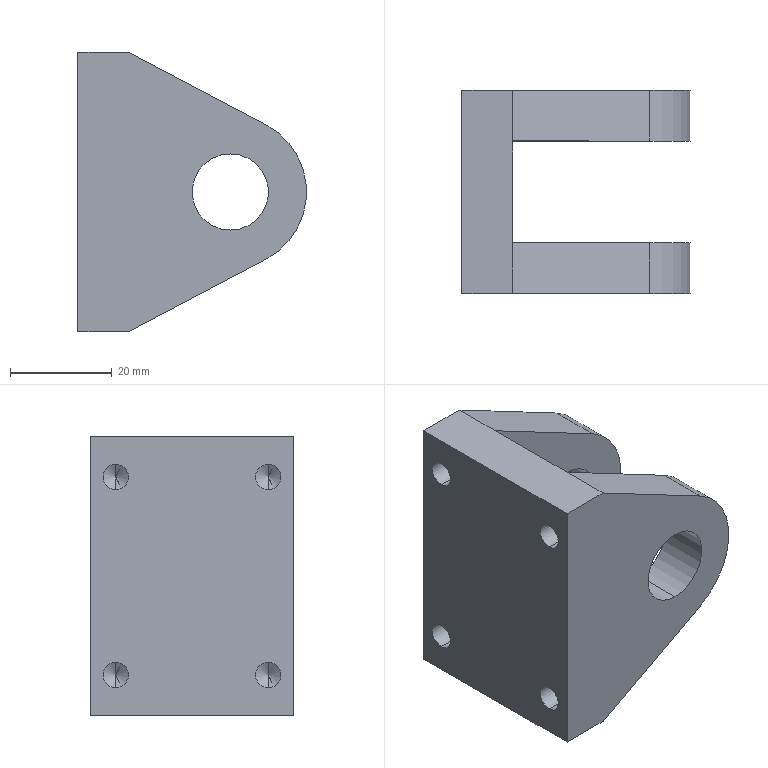Part | SolidWorks | features Chamfer 1, Extrusion 1, HoleWzd 1, ICE 1 | 1 solid | 34 faces | box 45 x 40 x 55 mm | volume 42289 mm3 | cylinder 14 | plane 12 | cone 8 | commonest cylinder face diameters 5 x8 15 x4 30 x2
STEP:
#1=CARTESIAN_POINT('',(15.,5.,-22.));
#2=VERTEX_POINT('',#1);
#3=CARTESIAN_POINT('',(15.,5.,-17.));
#4=VERTEX_POINT('',#3);
#5=CARTESIAN_POINT('',(15.,5.,-19.5));
#6=DIRECTION('',(-1.,0.,0.));
#7=DIRECTION('',(0.,0.,1.));
#8=AXIS2_PLACEMENT_3D('',#5,#6,#7);
#9=CIRCLE('',#8,2.5);
#10=EDGE_CURVE('',#2,#4,#9,.T.);
#11=ORIENTED_EDGE('',*,*,#10,.F.);
#12=CARTESIAN_POINT('',(0.,5.,-22.));
#13=VERTEX_POINT('',#12);
#14=CARTESIAN_POINT('',(0.,5.,-22.));
#15=DIRECTION('',(-1.,0.,0.));
#16=VECTOR('',#15,1000.);
#17=LINE('',#14,#16);
#18=EDGE_CURVE('',#2,#13,#17,.T.);
#19=ORIENTED_EDGE('',*,*,#18,.T.);
#20=CARTESIAN_POINT('',(0.,5.,-17.));
#21=VERTEX_POINT('',#20);
#22=CARTESIAN_POINT('',(0.,5.,-19.5));
#23=DIRECTION('',(-1.,0.,0.));
#24=DIRECTION('',(0.,0.,1.));
#25=AXIS2_PLACEMENT_3D('',#22,#23,#24);
#26=CIRCLE('',#25,2.5);
#27=EDGE_CURVE('',#13,#21,#26,.T.);
#28=ORIENTED_EDGE('',*,*,#27,.T.);
#29=CARTESIAN_POINT('',(0.,5.,-17.));
#30=DIRECTION('',(-1.,0.,0.));
#31=VECTOR('',#30,1000.);
#32=LINE('',#29,#31);
#33=EDGE_CURVE('',#4,#21,#32,.T.);
#34=ORIENTED_EDGE('',*,*,#33,.F.);
#35=EDGE_LOOP('',(#11,#19,#28,#34));
#36=FACE_OUTER_BOUND('',#35,.T.);
#37=CARTESIAN_POINT('',(0.,5.,-19.5));
#38=DIRECTION('',(-1.,0.,0.));
#39=DIRECTION('',(0.,0.,1.));
#40=AXIS2_PLACEMENT_3D('',#37,#38,#39);
#41=CYLINDRICAL_SURFACE('',#40,2.5);
#42=ADVANCED_FACE('',(#36),#41,.F.);
#43=CARTESIAN_POINT('',(16.502,5.,-19.5));
#44=VERTEX_POINT('',#43);
#45=CARTESIAN_POINT('',(15.,5.,-17.));
#46=DIRECTION('',(-0.515,0.,0.8572));
#47=VECTOR('',#46,1000.);
#48=LINE('',#45,#47);
#49=EDGE_CURVE('',#44,#4,#48,.T.);
#50=ORIENTED_EDGE('',*,*,#49,.F.);
#51=CARTESIAN_POINT('',(15.,5.,-22.));
#52=DIRECTION('',(-0.515,0.,-0.8572));
#53=VECTOR('',#52,1000.);
#54=LINE('',#51,#53);
#55=EDGE_CURVE('',#44,#2,#54,.T.);
#56=ORIENTED_EDGE('',*,*,#55,.T.);
#57=ORIENTED_EDGE('',*,*,#10,.T.);
#58=EDGE_LOOP('',(#50,#56,#57));
#59=FACE_OUTER_BOUND('',#58,.T.);
#60=CARTESIAN_POINT('',(15.,5.,-19.5));
#61=DIRECTION('',(-1.,0.,0.));
#62=DIRECTION('',(0.,0.,1.));
#63=AXIS2_PLACEMENT_3D('',#60,#61,#62);
#64=CONICAL_SURFACE('',#63,2.5,1.03);
#65=ADVANCED_FACE('',(#59),#64,.F.);
#66=CARTESIAN_POINT('',(15.,35.,-22.));
#67=VERTEX_POINT('',#66);
#68=CARTESIAN_POINT('',(15.,35.,-17.));
#69=VERTEX_POINT('',#68);
#70=CARTESIAN_POINT('',(15.,35.,-19.5));
#71=DIRECTION('',(-1.,0.,0.));
#72=DIRECTION('',(0.,0.,1.));
#73=AXIS2_PLACEMENT_3D('',#70,#71,#72);
#74=CIRCLE('',#73,2.5);
#75=EDGE_CURVE('',#67,#69,#74,.T.);
#76=ORIENTED_EDGE('',*,*,#75,.F.);
#77=CARTESIAN_POINT('',(0.,35.,-22.));
#78=VERTEX_POINT('',#77);
#79=CARTESIAN_POINT('',(0.,35.,-22.));
#80=DIRECTION('',(-1.,0.,0.));
#81=VECTOR('',#80,1000.);
#82=LINE('',#79,#81);
#83=EDGE_CURVE('',#67,#78,#82,.T.);
#84=ORIENTED_EDGE('',*,*,#83,.T.);
#85=CARTESIAN_POINT('',(0.,35.,-17.));
#86=VERTEX_POINT('',#85);
#87=CARTESIAN_POINT('',(0.,35.,-19.5));
#88=DIRECTION('',(-1.,0.,0.));
#89=DIRECTION('',(0.,0.,1.));
#90=AXIS2_PLACEMENT_3D('',#87,#88,#89);
#91=CIRCLE('',#90,2.5);
#92=EDGE_CURVE('',#78,#86,#91,.T.);
#93=ORIENTED_EDGE('',*,*,#92,.T.);
#94=CARTESIAN_POINT('',(0.,35.,-17.));
#95=DIRECTION('',(-1.,0.,0.));
#96=VECTOR('',#95,1000.);
#97=LINE('',#94,#96);
#98=EDGE_CURVE('',#69,#86,#97,.T.);
#99=ORIENTED_EDGE('',*,*,#98,.F.);
#100=EDGE_LOOP('',(#76,#84,#93,#99));
#101=FACE_OUTER_BOUND('',#100,.T.);
#102=CARTESIAN_POINT('',(0.,35.,-19.5));
#103=DIRECTION('',(-1.,0.,0.));
#104=DIRECTION('',(0.,0.,1.));
#105=AXIS2_PLACEMENT_3D('',#102,#103,#104);
#106=CYLINDRICAL_SURFACE('',#105,2.5);
#107=ADVANCED_FACE('',(#101),#106,.F.);
#108=CARTESIAN_POINT('',(16.502,35.,-19.5));
#109=VERTEX_POINT('',#108);
#110=CARTESIAN_POINT('',(15.,35.,-17.));
#111=DIRECTION('',(-0.515,0.,0.8572));
#112=VECTOR('',#111,1000.);
#113=LINE('',#110,#112);
#114=EDGE_CURVE('',#109,#69,#113,.T.);
#115=ORIENTED_EDGE('',*,*,#114,.F.);
#116=CARTESIAN_POINT('',(15.,35.,-22.));
#117=DIRECTION('',(-0.515,0.,-0.8572));
#118=VECTOR('',#117,1000.);
#119=LINE('',#116,#118);
#120=EDGE_CURVE('',#109,#67,#119,.T.);
#121=ORIENTED_EDGE('',*,*,#120,.T.);
#122=ORIENTED_EDGE('',*,*,#75,.T.);
#123=EDGE_LOOP('',(#115,#121,#122));
#124=FACE_OUTER_BOUND('',#123,.T.);
#125=CARTESIAN_POINT('',(15.,35.,-19.5));
#126=DIRECTION('',(-1.,0.,0.));
#127=DIRECTION('',(0.,0.,1.));
#128=AXIS2_PLACEMENT_3D('',#125,#126,#127);
#129=CONICAL_SURFACE('',#128,2.5,1.03);
#130=ADVANCED_FACE('',(#124),#129,.F.);
#131=CARTESIAN_POINT('',(15.,5.,17.));
#132=VERTEX_POINT('',#131);
#133=CARTESIAN_POINT('',(15.,5.,22.));
#134=VERTEX_POINT('',#133);
#135=CARTESIAN_POINT('',(15.,5.,19.5));
#136=DIRECTION('',(-1.,0.,0.));
#137=DIRECTION('',(0.,0.,1.));
#138=AXIS2_PLACEMENT_3D('',#135,#136,#137);
#139=CIRCLE('',#138,2.5);
#140=EDGE_CURVE('',#132,#134,#139,.T.);
#141=ORIENTED_EDGE('',*,*,#140,.F.);
#142=CARTESIAN_POINT('',(0.,5.,17.));
#143=VERTEX_POINT('',#142);
#144=CARTESIAN_POINT('',(0.,5.,17.));
#145=DIRECTION('',(-1.,0.,0.));
#146=VECTOR('',#145,1000.);
#147=LINE('',#144,#146);
#148=EDGE_CURVE('',#132,#143,#147,.T.);
#149=ORIENTED_EDGE('',*,*,#148,.T.);
#150=CARTESIAN_POINT('',(0.,5.,22.));
#151=VERTEX_POINT('',#150);
#152=CARTESIAN_POINT('',(0.,5.,19.5));
#153=DIRECTION('',(-1.,0.,0.));
#154=DIRECTION('',(0.,0.,1.));
#155=AXIS2_PLACEMENT_3D('',#152,#153,#154);
#156=CIRCLE('',#155,2.5);
#157=EDGE_CURVE('',#143,#151,#156,.T.);
#158=ORIENTED_EDGE('',*,*,#157,.T.);
#159=CARTESIAN_POINT('',(0.,5.,22.));
#160=DIRECTION('',(-1.,0.,0.));
#161=VECTOR('',#160,1000.);
#162=LINE('',#159,#161);
#163=EDGE_CURVE('',#134,#151,#162,.T.);
#164=ORIENTED_EDGE('',*,*,#163,.F.);
#165=EDGE_LOOP('',(#141,#149,#158,#164));
#166=FACE_OUTER_BOUND('',#165,.T.);
#167=CARTESIAN_POINT('',(0.,5.,19.5));
#168=DIRECTION('',(-1.,0.,0.));
#169=DIRECTION('',(0.,0.,1.));
#170=AXIS2_PLACEMENT_3D('',#167,#168,#169);
#171=CYLINDRICAL_SURFACE('',#170,2.5);
#172=ADVANCED_FACE('',(#166),#171,.F.);
#173=CARTESIAN_POINT('',(16.502,5.,19.5));
#174=VERTEX_POINT('',#173);
#175=CARTESIAN_POINT('',(15.,5.,22.));
#176=DIRECTION('',(-0.515,0.,0.8572));
#177=VECTOR('',#176,1000.);
#178=LINE('',#175,#177);
#179=EDGE_CURVE('',#174,#134,#178,.T.);
#180=ORIENTED_EDGE('',*,*,#179,.F.);
#181=CARTESIAN_POINT('',(15.,5.,17.));
#182=DIRECTION('',(-0.515,0.,-0.8572));
#183=VECTOR('',#182,1000.);
#184=LINE('',#181,#183);
#185=EDGE_CURVE('',#174,#132,#184,.T.);
#186=ORIENTED_EDGE('',*,*,#185,.T.);
#187=ORIENTED_EDGE('',*,*,#140,.T.);
#188=EDGE_LOOP('',(#180,#186,#187));
#189=FACE_OUTER_BOUND('',#188,.T.);
#190=CARTESIAN_POINT('',(15.,5.,19.5));
#191=DIRECTION('',(-1.,0.,0.));
#192=DIRECTION('',(0.,0.,1.));
#193=AXIS2_PLACEMENT_3D('',#190,#191,#192);
#194=CONICAL_SURFACE('',#193,2.5,1.03);
#195=ADVANCED_FACE('',(#189),#194,.F.);
#196=CARTESIAN_POINT('',(15.,35.,17.));
#197=VERTEX_POINT('',#196);
#198=CARTESIAN_POINT('',(15.,35.,22.));
#199=VERTEX_POINT('',#198);
#200=CARTESIAN_POINT('',(15.,35.,19.5));
#201=DIRECTION('',(-1.,0.,0.));
#202=DIRECTION('',(0.,0.,1.));
#203=AXIS2_PLACEMENT_3D('',#200,#201,#202);
#204=CIRCLE('',#203,2.5);
#205=EDGE_CURVE('',#197,#199,#204,.T.);
#206=ORIENTED_EDGE('',*,*,#205,.F.);
#207=CARTESIAN_POINT('',(0.,35.,17.));
#208=VERTEX_POINT('',#207);
#209=CARTESIAN_POINT('',(0.,35.,17.));
#210=DIRECTION('',(-1.,0.,0.));
#211=VECTOR('',#210,1000.);
#212=LINE('',#209,#211);
#213=EDGE_CURVE('',#197,#208,#212,.T.);
#214=ORIENTED_EDGE('',*,*,#213,.T.);
#215=CARTESIAN_POINT('',(0.,35.,22.));
#216=VERTEX_POINT('',#215);
#217=CARTESIAN_POINT('',(0.,35.,19.5));
#218=DIRECTION('',(-1.,0.,0.));
#219=DIRECTION('',(0.,0.,1.));
#220=AXIS2_PLACEMENT_3D('',#217,#218,#219);
#221=CIRCLE('',#220,2.5);
#222=EDGE_CURVE('',#208,#216,#221,.T.);
#223=ORIENTED_EDGE('',*,*,#222,.T.);
#224=CARTESIAN_POINT('',(0.,35.,22.));
#225=DIRECTION('',(-1.,0.,0.));
#226=VECTOR('',#225,1000.);
#227=LINE('',#224,#226);
#228=EDGE_CURVE('',#199,#216,#227,.T.);
#229=ORIENTED_EDGE('',*,*,#228,.F.);
#230=EDGE_LOOP('',(#206,#214,#223,#229));
#231=FACE_OUTER_BOUND('',#230,.T.);
#232=CARTESIAN_POINT('',(0.,35.,19.5));
#233=DIRECTION('',(-1.,0.,0.));
#234=DIRECTION('',(0.,0.,1.));
#235=AXIS2_PLACEMENT_3D('',#232,#233,#234);
#236=CYLINDRICAL_SURFACE('',#235,2.5);
#237=ADVANCED_FACE('',(#231),#236,.F.);
#238=CARTESIAN_POINT('',(16.502,35.,19.5));
#239=VERTEX_POINT('',#238);
#240=CARTESIAN_POINT('',(15.,35.,22.));
#241=DIRECTION('',(-0.515,0.,0.8572));
#242=VECTOR('',#241,1000.);
#243=LINE('',#240,#242);
#244=EDGE_CURVE('',#239,#199,#243,.T.);
#245=ORIENTED_EDGE('',*,*,#244,.F.);
#246=CARTESIAN_POINT('',(15.,35.,17.));
#247=DIRECTION('',(-0.515,0.,-0.8572));
#248=VECTOR('',#247,1000.);
#249=LINE('',#246,#248);
#250=EDGE_CURVE('',#239,#197,#249,.T.);
#251=ORIENTED_EDGE('',*,*,#250,.T.);
#252=ORIENTED_EDGE('',*,*,#205,.T.);
#253=EDGE_LOOP('',(#245,#251,#252));
#254=FACE_OUTER_BOUND('',#253,.T.);
#255=CARTESIAN_POINT('',(15.,35.,19.5));
#256=DIRECTION('',(-1.,0.,0.));
#257=DIRECTION('',(0.,0.,1.));
#258=AXIS2_PLACEMENT_3D('',#255,#256,#257);
#259=CONICAL_SURFACE('',#258,2.5,1.03);
#260=ADVANCED_FACE('',(#254),#259,.F.);
#261=CARTESIAN_POINT('',(30.,40.,-7.5));
#262=VERTEX_POINT('',#261);
#263=CARTESIAN_POINT('',(30.,40.,7.5));
#264=VERTEX_POINT('',#263);
#265=CARTESIAN_POINT('',(30.,40.,0.));
#266=DIRECTION('',(0.,1.,0.));
#267=DIRECTION('',(0.,0.,1.));
#268=AXIS2_PLACEMENT_3D('',#265,#266,#267);
#269=CIRCLE('',#268,7.5);
#270=EDGE_CURVE('',#262,#264,#269,.T.);
#271=ORIENTED_EDGE('',*,*,#270,.T.);
#272=CARTESIAN_POINT('',(30.,30.,7.5));
#273=VERTEX_POINT('',#272);
#274=CARTESIAN_POINT('',(30.,40.,7.5));
#275=DIRECTION('',(0.,-1.,0.));
#276=VECTOR('',#275,1000.);
#277=LINE('',#274,#276);
#278=EDGE_CURVE('',#264,#273,#277,.T.);
#279=ORIENTED_EDGE('',*,*,#278,.T.);
#280=CARTESIAN_POINT('',(30.,30.,-7.5));
#281=VERTEX_POINT('',#280);
#282=CARTESIAN_POINT('',(30.,30.,0.));
#283=DIRECTION('',(0.,1.,0.));
#284=DIRECTION('',(-1.,0.,0.));
#285=AXIS2_PLACEMENT_3D('',#282,#283,#284);
#286=CIRCLE('',#285,7.5);
#287=EDGE_CURVE('',#281,#273,#286,.T.);
#288=ORIENTED_EDGE('',*,*,#287,.F.);
#289=CARTESIAN_POINT('',(30.,40.,-7.5));
#290=DIRECTION('',(0.,-1.,0.));
#291=VECTOR('',#290,1000.);
#292=LINE('',#289,#291);
#293=EDGE_CURVE('',#262,#281,#292,.T.);
#294=ORIENTED_EDGE('',*,*,#293,.F.);
#295=EDGE_LOOP('',(#271,#279,#288,#294));
#296=FACE_OUTER_BOUND('',#295,.T.);
#297=CARTESIAN_POINT('',(30.,40.,0.));
#298=DIRECTION('',(0.,-1.,0.));
#299=DIRECTION('',(0.,0.,-1.));
#300=AXIS2_PLACEMENT_3D('',#297,#298,#299);
#301=CYLINDRICAL_SURFACE('',#300,7.5);
#302=ADVANCED_FACE('',(#296),#301,.F.);
#303=CARTESIAN_POINT('',(30.,10.,7.5));
#304=VERTEX_POINT('',#303);
#305=CARTESIAN_POINT('',(30.,10.,-7.5));
#306=VERTEX_POINT('',#305);
#307=CARTESIAN_POINT('',(30.,10.,0.));
#308=DIRECTION('',(0.,-1.,0.));
#309=DIRECTION('',(1.,0.,0.));
#310=AXIS2_PLACEMENT_3D('',#307,#308,#309);
#311=CIRCLE('',#310,7.5);
#312=EDGE_CURVE('',#304,#306,#311,.T.);
#313=ORIENTED_EDGE('',*,*,#312,.F.);
#314=CARTESIAN_POINT('',(30.,0.,7.5));
#315=VERTEX_POINT('',#314);
#316=CARTESIAN_POINT('',(30.,40.,7.5));
#317=DIRECTION('',(0.,-1.,0.));
#318=VECTOR('',#317,1000.);
#319=LINE('',#316,#318);
#320=EDGE_CURVE('',#304,#315,#319,.T.);
#321=ORIENTED_EDGE('',*,*,#320,.T.);
#322=CARTESIAN_POINT('',(30.,0.,-7.5));
#323=VERTEX_POINT('',#322);
#324=CARTESIAN_POINT('',(30.,0.,0.));
#325=DIRECTION('',(0.,1.,0.));
#326=DIRECTION('',(0.,0.,1.));
#327=AXIS2_PLACEMENT_3D('',#324,#325,#326);
#328=CIRCLE('',#327,7.5);
#329=EDGE_CURVE('',#323,#315,#328,.T.);
#330=ORIENTED_EDGE('',*,*,#329,.F.);
#331=CARTESIAN_POINT('',(30.,40.,-7.5));
#332=DIRECTION('',(0.,-1.,0.));
#333=VECTOR('',#332,1000.);
#334=LINE('',#331,#333);
#335=EDGE_CURVE('',#306,#323,#334,.T.);
#336=ORIENTED_EDGE('',*,*,#335,.F.);
#337=EDGE_LOOP('',(#313,#321,#330,#336));
#338=FACE_OUTER_BOUND('',#337,.T.);
#339=CARTESIAN_POINT('',(30.,40.,0.));
#340=DIRECTION('',(0.,-1.,0.));
#341=DIRECTION('',(0.,0.,-1.));
#342=AXIS2_PLACEMENT_3D('',#339,#340,#341);
#343=CYLINDRICAL_SURFACE('',#342,7.5);
#344=ADVANCED_FACE('',(#338),#343,.F.);
#345=CARTESIAN_POINT('',(36.995,10.,13.269));
#346=VERTEX_POINT('',#345);
#347=CARTESIAN_POINT('',(36.995,0.,13.269));
#348=VERTEX_POINT('',#347);
#349=CARTESIAN_POINT('',(36.995,40.,13.269));
#350=DIRECTION('',(0.,-1.,0.));
#351=VECTOR('',#350,1000.);
#352=LINE('',#349,#351);
#353=EDGE_CURVE('',#346,#348,#352,.T.);
#354=ORIENTED_EDGE('',*,*,#353,.F.);
#355=CARTESIAN_POINT('',(10.,10.,27.5));
#356=VERTEX_POINT('',#355);
#357=CARTESIAN_POINT('',(10.,10.,27.5));
#358=DIRECTION('',(-0.8846,0.,0.4663));
#359=VECTOR('',#358,1000.);
#360=LINE('',#357,#359);
#361=EDGE_CURVE('',#346,#356,#360,.T.);
#362=ORIENTED_EDGE('',*,*,#361,.T.);
#363=CARTESIAN_POINT('',(10.,0.,27.5));
#364=VERTEX_POINT('',#363);
#365=CARTESIAN_POINT('',(10.,40.,27.5));
#366=DIRECTION('',(0.,-1.,0.));
#367=VECTOR('',#366,1000.);
#368=LINE('',#365,#367);
#369=EDGE_CURVE('',#356,#364,#368,.T.);
#370=ORIENTED_EDGE('',*,*,#369,.T.);
#371=CARTESIAN_POINT('',(10.,0.,27.5));
#372=DIRECTION('',(0.8846,0.,-0.4663));
#373=VECTOR('',#372,1000.);
#374=LINE('',#371,#373);
#375=EDGE_CURVE('',#364,#348,#374,.T.);
#376=ORIENTED_EDGE('',*,*,#375,.T.);
#377=EDGE_LOOP('',(#354,#362,#370,#376));
#378=FACE_OUTER_BOUND('',#377,.T.);
#379=CARTESIAN_POINT('',(10.,40.,27.5));
#380=DIRECTION('',(-0.4663,0.,-0.8846));
#381=DIRECTION('',(-0.8846,0.,0.4663));
#382=AXIS2_PLACEMENT_3D('',#379,#380,#381);
#383=PLANE('',#382);
#384=ADVANCED_FACE('',(#378),#383,.F.);
#385=CARTESIAN_POINT('',(36.995,10.,-13.269));
#386=VERTEX_POINT('',#385);
#387=CARTESIAN_POINT('',(36.995,0.,-13.269));
#388=VERTEX_POINT('',#387);
#389=CARTESIAN_POINT('',(36.995,40.,-13.269));
#390=DIRECTION('',(0.,-1.,0.));
#391=VECTOR('',#390,1000.);
#392=LINE('',#389,#391);
#393=EDGE_CURVE('',#386,#388,#392,.T.);
#394=ORIENTED_EDGE('',*,*,#393,.F.);
#395=CARTESIAN_POINT('',(30.,10.,0.));
#396=DIRECTION('',(0.,-1.,0.));
#397=DIRECTION('',(1.,0.,0.));
#398=AXIS2_PLACEMENT_3D('',#395,#396,#397);
#399=CIRCLE('',#398,15.);
#400=EDGE_CURVE('',#386,#346,#399,.T.);
#401=ORIENTED_EDGE('',*,*,#400,.T.);
#402=ORIENTED_EDGE('',*,*,#353,.T.);
#403=CARTESIAN_POINT('',(30.,0.,0.));
#404=DIRECTION('',(0.,1.,0.));
#405=DIRECTION('',(0.,0.,1.));
#406=AXIS2_PLACEMENT_3D('',#403,#404,#405);
#407=CIRCLE('',#406,15.);
#408=EDGE_CURVE('',#348,#388,#407,.T.);
#409=ORIENTED_EDGE('',*,*,#408,.T.);
#410=EDGE_LOOP('',(#394,#401,#402,#409));
#411=FACE_OUTER_BOUND('',#410,.T.);
#412=CARTESIAN_POINT('',(30.,40.,0.));
#413=DIRECTION('',(0.,-1.,0.));
#414=DIRECTION('',(0.,0.,-1.));
#415=AXIS2_PLACEMENT_3D('',#412,#413,#414);
#416=CYLINDRICAL_SURFACE('',#415,15.);
#417=ADVANCED_FACE('',(#411),#416,.T.);
#418=CARTESIAN_POINT('',(10.,10.,-27.5));
#419=VERTEX_POINT('',#418);
#420=CARTESIAN_POINT('',(10.,0.,-27.5));
#421=VERTEX_POINT('',#420);
#422=CARTESIAN_POINT('',(10.,40.,-27.5));
#423=DIRECTION('',(0.,-1.,0.));
#424=VECTOR('',#423,1000.);
#425=LINE('',#422,#424);
#426=EDGE_CURVE('',#419,#421,#425,.T.);
#427=ORIENTED_EDGE('',*,*,#426,.F.);
#428=CARTESIAN_POINT('',(10.,10.,-27.5));
#429=DIRECTION('',(0.8846,0.,0.4663));
#430=VECTOR('',#429,1000.);
#431=LINE('',#428,#430);
#432=EDGE_CURVE('',#419,#386,#431,.T.);
#433=ORIENTED_EDGE('',*,*,#432,.T.);
#434=ORIENTED_EDGE('',*,*,#393,.T.);
#435=CARTESIAN_POINT('',(10.,0.,-27.5));
#436=DIRECTION('',(-0.8846,0.,-0.4663));
#437=VECTOR('',#436,1000.);
#438=LINE('',#435,#437);
#439=EDGE_CURVE('',#388,#421,#438,.T.);
#440=ORIENTED_EDGE('',*,*,#439,.T.);
#441=EDGE_LOOP('',(#427,#433,#434,#440));
#442=FACE_OUTER_BOUND('',#441,.T.);
#443=CARTESIAN_POINT('',(10.,40.,-27.5));
#444=DIRECTION('',(-0.4663,0.,0.8846));
#445=DIRECTION('',(0.8846,0.,0.4663));
#446=AXIS2_PLACEMENT_3D('',#443,#444,#445);
#447=PLANE('',#446);
#448=ADVANCED_FACE('',(#442),#447,.F.);
#449=ORIENTED_EDGE('',*,*,#320,.F.);
#450=CARTESIAN_POINT('',(30.,10.,0.));
#451=DIRECTION('',(0.,-1.,0.));
#452=DIRECTION('',(1.,0.,0.));
#453=AXIS2_PLACEMENT_3D('',#450,#451,#452);
#454=CIRCLE('',#453,7.5);
#455=EDGE_CURVE('',#306,#304,#454,.T.);
#456=ORIENTED_EDGE('',*,*,#455,.F.);
#457=ORIENTED_EDGE('',*,*,#335,.T.);
#458=CARTESIAN_POINT('',(30.,0.,0.));
#459=DIRECTION('',(0.,1.,0.));
#460=DIRECTION('',(0.,0.,1.));
#461=AXIS2_PLACEMENT_3D('',#458,#459,#460);
#462=CIRCLE('',#461,7.5);
#463=EDGE_CURVE('',#315,#323,#462,.T.);
#464=ORIENTED_EDGE('',*,*,#463,.F.);
#465=EDGE_LOOP('',(#449,#456,#457,#464));
#466=FACE_OUTER_BOUND('',#465,.T.);
#467=CARTESIAN_POINT('',(30.,40.,0.));
#468=DIRECTION('',(0.,-1.,0.));
#469=DIRECTION('',(0.,0.,-1.));
#470=AXIS2_PLACEMENT_3D('',#467,#468,#469);
#471=CYLINDRICAL_SURFACE('',#470,7.5);
#472=ADVANCED_FACE('',(#466),#471,.F.);
#473=CARTESIAN_POINT('',(10.,40.,-27.5));
#474=VERTEX_POINT('',#473);
#475=CARTESIAN_POINT('',(0.,40.,-27.5));
#476=VERTEX_POINT('',#475);
#477=CARTESIAN_POINT('',(0.,40.,-27.5));
#478=DIRECTION('',(-1.,0.,0.));
#479=VECTOR('',#478,1000.);
#480=LINE('',#477,#479);
#481=EDGE_CURVE('',#474,#476,#480,.T.);
#482=ORIENTED_EDGE('',*,*,#481,.T.);
#483=CARTESIAN_POINT('',(0.,40.,27.5));
#484=VERTEX_POINT('',#483);
#485=CARTESIAN_POINT('',(0.,40.,27.5));
#486=DIRECTION('',(0.,0.,1.));
#487=VECTOR('',#486,1000.);
#488=LINE('',#485,#487);
#489=EDGE_CURVE('',#476,#484,#488,.T.);
#490=ORIENTED_EDGE('',*,*,#489,.T.);
#491=CARTESIAN_POINT('',(10.,40.,27.5));
#492=VERTEX_POINT('',#491);
#493=CARTESIAN_POINT('',(0.,40.,27.5));
#494=DIRECTION('',(1.,0.,0.));
#495=VECTOR('',#494,1000.);
#496=LINE('',#493,#495);
#497=EDGE_CURVE('',#484,#492,#496,.T.);
#498=ORIENTED_EDGE('',*,*,#497,.T.);
#499=CARTESIAN_POINT('',(36.995,40.,13.269));
#500=VERTEX_POINT('',#499);
#501=CARTESIAN_POINT('',(10.,40.,27.5));
#502=DIRECTION('',(0.8846,0.,-0.4663));
#503=VECTOR('',#502,1000.);
#504=LINE('',#501,#503);
#505=EDGE_CURVE('',#492,#500,#504,.T.);
#506=ORIENTED_EDGE('',*,*,#505,.T.);
#507=CARTESIAN_POINT('',(36.995,40.,-13.269));
#508=VERTEX_POINT('',#507);
#509=CARTESIAN_POINT('',(30.,40.,0.));
#510=DIRECTION('',(0.,1.,0.));
#511=DIRECTION('',(0.,0.,1.));
#512=AXIS2_PLACEMENT_3D('',#509,#510,#511);
#513=CIRCLE('',#512,15.);
#514=EDGE_CURVE('',#500,#508,#513,.T.);
#515=ORIENTED_EDGE('',*,*,#514,.T.);
#516=CARTESIAN_POINT('',(10.,40.,-27.5));
#517=DIRECTION('',(-0.8846,0.,-0.4663));
#518=VECTOR('',#517,1000.);
#519=LINE('',#516,#518);
#520=EDGE_CURVE('',#508,#474,#519,.T.);
#521=ORIENTED_EDGE('',*,*,#520,.T.);
#522=EDGE_LOOP('',(#482,#490,#498,#506,#515,#521));
#523=FACE_OUTER_BOUND('',#522,.T.);
#524=ORIENTED_EDGE('',*,*,#270,.F.);
#525=CARTESIAN_POINT('',(30.,40.,0.));
#526=DIRECTION('',(0.,1.,0.));
#527=DIRECTION('',(0.,0.,1.));
#528=AXIS2_PLACEMENT_3D('',#525,#526,#527);
#529=CIRCLE('',#528,7.5);
#530=EDGE_CURVE('',#264,#262,#529,.T.);
#531=ORIENTED_EDGE('',*,*,#530,.F.);
#532=EDGE_LOOP('',(#524,#531));
#533=FACE_BOUND('',#532,.T.);
#534=CARTESIAN_POINT('',(30.,40.,0.));
#535=DIRECTION('',(0.,1.,0.));
#536=DIRECTION('',(0.,0.,1.));
#537=AXIS2_PLACEMENT_3D('',#534,#535,#536);
#538=PLANE('',#537);
#539=ADVANCED_FACE('',(#523,#533),#538,.T.);
#540=CARTESIAN_POINT('',(0.,0.,-27.5));
#541=VERTEX_POINT('',#540);
#542=CARTESIAN_POINT('',(0.,0.,-27.5));
#543=DIRECTION('',(-1.,0.,0.));
#544=VECTOR('',#543,1000.);
#545=LINE('',#542,#544);
#546=EDGE_CURVE('',#421,#541,#545,.T.);
#547=ORIENTED_EDGE('',*,*,#546,.F.);
#548=ORIENTED_EDGE('',*,*,#439,.F.);
#549=ORIENTED_EDGE('',*,*,#408,.F.);
#550=ORIENTED_EDGE('',*,*,#375,.F.);
#551=CARTESIAN_POINT('',(0.,0.,27.5));
#552=VERTEX_POINT('',#551);
#553=CARTESIAN_POINT('',(0.,0.,27.5));
#554=DIRECTION('',(1.,0.,0.));
#555=VECTOR('',#554,1000.);
#556=LINE('',#553,#555);
#557=EDGE_CURVE('',#552,#364,#556,.T.);
#558=ORIENTED_EDGE('',*,*,#557,.F.);
#559=CARTESIAN_POINT('',(0.,0.,27.5));
#560=DIRECTION('',(0.,0.,1.));
#561=VECTOR('',#560,1000.);
#562=LINE('',#559,#561);
#563=EDGE_CURVE('',#541,#552,#562,.T.);
#564=ORIENTED_EDGE('',*,*,#563,.F.);
#565=EDGE_LOOP('',(#547,#548,#549,#550,#558,#564));
#566=FACE_OUTER_BOUND('',#565,.T.);
#567=ORIENTED_EDGE('',*,*,#329,.T.);
#568=ORIENTED_EDGE('',*,*,#463,.T.);
#569=EDGE_LOOP('',(#567,#568));
#570=FACE_BOUND('',#569,.T.);
#571=CARTESIAN_POINT('',(30.,0.,0.));
#572=DIRECTION('',(0.,1.,0.));
#573=DIRECTION('',(0.,0.,1.));
#574=AXIS2_PLACEMENT_3D('',#571,#572,#573);
#575=PLANE('',#574);
#576=ADVANCED_FACE('',(#566,#570),#575,.F.);
#577=ORIENTED_EDGE('',*,*,#546,.T.);
#578=CARTESIAN_POINT('',(0.,40.,-27.5));
#579=DIRECTION('',(0.,-1.,0.));
#580=VECTOR('',#579,1000.);
#581=LINE('',#578,#580);
#582=EDGE_CURVE('',#476,#541,#581,.T.);
#583=ORIENTED_EDGE('',*,*,#582,.F.);
#584=ORIENTED_EDGE('',*,*,#481,.F.);
#585=CARTESIAN_POINT('',(10.,30.,-27.5));
#586=VERTEX_POINT('',#585);
#587=CARTESIAN_POINT('',(10.,40.,-27.5));
#588=DIRECTION('',(0.,-1.,0.));
#589=VECTOR('',#588,1000.);
#590=LINE('',#587,#589);
#591=EDGE_CURVE('',#474,#586,#590,.T.);
#592=ORIENTED_EDGE('',*,*,#591,.T.);
#593=CARTESIAN_POINT('',(10.,30.,-27.5));
#594=DIRECTION('',(0.,1.,0.));
#595=VECTOR('',#594,1000.);
#596=LINE('',#593,#595);
#597=EDGE_CURVE('',#419,#586,#596,.T.);
#598=ORIENTED_EDGE('',*,*,#597,.F.);
#599=ORIENTED_EDGE('',*,*,#426,.T.);
#600=EDGE_LOOP('',(#577,#583,#584,#592,#598,#599));
#601=FACE_OUTER_BOUND('',#600,.T.);
#602=CARTESIAN_POINT('',(0.,40.,-27.5));
#603=DIRECTION('',(0.,0.,1.));
#604=DIRECTION('',(1.,0.,0.));
#605=AXIS2_PLACEMENT_3D('',#602,#603,#604);
#606=PLANE('',#605);
#607=ADVANCED_FACE('',(#601),#606,.F.);
#608=CARTESIAN_POINT('',(0.,5.,-19.5));
#609=DIRECTION('',(-1.,0.,0.));
#610=DIRECTION('',(0.,0.,1.));
#611=AXIS2_PLACEMENT_3D('',#608,#609,#610);
#612=CIRCLE('',#611,2.5);
#613=EDGE_CURVE('',#21,#13,#612,.T.);
#614=ORIENTED_EDGE('',*,*,#613,.F.);
#615=ORIENTED_EDGE('',*,*,#27,.F.);
#616=EDGE_LOOP('',(#614,#615));
#617=FACE_BOUND('',#616,.T.);
#618=CARTESIAN_POINT('',(0.,35.,-19.5));
#619=DIRECTION('',(-1.,0.,0.));
#620=DIRECTION('',(0.,0.,1.));
#621=AXIS2_PLACEMENT_3D('',#618,#619,#620);
#622=CIRCLE('',#621,2.5);
#623=EDGE_CURVE('',#86,#78,#622,.T.);
#624=ORIENTED_EDGE('',*,*,#623,.F.);
#625=ORIENTED_EDGE('',*,*,#92,.F.);
#626=EDGE_LOOP('',(#624,#625));
#627=FACE_BOUND('',#626,.T.);
#628=CARTESIAN_POINT('',(0.,5.,19.5));
#629=DIRECTION('',(-1.,0.,0.));
#630=DIRECTION('',(0.,0.,1.));
#631=AXIS2_PLACEMENT_3D('',#628,#629,#630);
#632=CIRCLE('',#631,2.5);
#633=EDGE_CURVE('',#151,#143,#632,.T.);
#634=ORIENTED_EDGE('',*,*,#633,.F.);
#635=ORIENTED_EDGE('',*,*,#157,.F.);
#636=EDGE_LOOP('',(#634,#635));
#637=FACE_BOUND('',#636,.T.);
#638=CARTESIAN_POINT('',(0.,35.,19.5));
#639=DIRECTION('',(-1.,0.,0.));
#640=DIRECTION('',(0.,0.,1.));
#641=AXIS2_PLACEMENT_3D('',#638,#639,#640);
#642=CIRCLE('',#641,2.5);
#643=EDGE_CURVE('',#216,#208,#642,.T.);
#644=ORIENTED_EDGE('',*,*,#643,.F.);
#645=ORIENTED_EDGE('',*,*,#222,.F.);
#646=EDGE_LOOP('',(#644,#645));
#647=FACE_BOUND('',#646,.T.);
#648=ORIENTED_EDGE('',*,*,#563,.T.);
#649=CARTESIAN_POINT('',(0.,40.,27.5));
#650=DIRECTION('',(0.,-1.,0.));
#651=VECTOR('',#650,1000.);
#652=LINE('',#649,#651);
#653=EDGE_CURVE('',#484,#552,#652,.T.);
#654=ORIENTED_EDGE('',*,*,#653,.F.);
#655=ORIENTED_EDGE('',*,*,#489,.F.);
#656=ORIENTED_EDGE('',*,*,#582,.T.);
#657=EDGE_LOOP('',(#648,#654,#655,#656));
#658=FACE_OUTER_BOUND('',#657,.T.);
#659=CARTESIAN_POINT('',(0.,40.,27.5));
#660=DIRECTION('',(1.,0.,0.));
#661=DIRECTION('',(0.,0.,-1.));
#662=AXIS2_PLACEMENT_3D('',#659,#660,#661);
#663=PLANE('',#662);
#664=ADVANCED_FACE('',(#617,#627,#637,#647,#658),#663,.F.);
#665=ORIENTED_EDGE('',*,*,#557,.T.);
#666=ORIENTED_EDGE('',*,*,#369,.F.);
#667=CARTESIAN_POINT('',(10.,30.,27.5));
#668=VERTEX_POINT('',#667);
#669=CARTESIAN_POINT('',(10.,30.,27.5));
#670=DIRECTION('',(0.,1.,0.));
#671=VECTOR('',#670,1000.);
#672=LINE('',#669,#671);
#673=EDGE_CURVE('',#356,#668,#672,.T.);
#674=ORIENTED_EDGE('',*,*,#673,.T.);
#675=CARTESIAN_POINT('',(10.,40.,27.5));
#676=DIRECTION('',(0.,-1.,0.));
#677=VECTOR('',#676,1000.);
#678=LINE('',#675,#677);
#679=EDGE_CURVE('',#492,#668,#678,.T.);
#680=ORIENTED_EDGE('',*,*,#679,.F.);
#681=ORIENTED_EDGE('',*,*,#497,.F.);
#682=ORIENTED_EDGE('',*,*,#653,.T.);
#683=EDGE_LOOP('',(#665,#666,#674,#680,#681,#682));
#684=FACE_OUTER_BOUND('',#683,.T.);
#685=CARTESIAN_POINT('',(0.,40.,27.5));
#686=DIRECTION('',(0.,0.,-1.));
#687=DIRECTION('',(-1.,0.,0.));
#688=AXIS2_PLACEMENT_3D('',#685,#686,#687);
#689=PLANE('',#688);
#690=ADVANCED_FACE('',(#684),#689,.F.);
#691=ORIENTED_EDGE('',*,*,#679,.T.);
#692=CARTESIAN_POINT('',(36.995,30.,13.269));
#693=VERTEX_POINT('',#692);
#694=CARTESIAN_POINT('',(10.,30.,27.5));
#695=DIRECTION('',(0.8846,0.,-0.4663));
#696=VECTOR('',#695,1000.);
#697=LINE('',#694,#696);
#698=EDGE_CURVE('',#668,#693,#697,.T.);
#699=ORIENTED_EDGE('',*,*,#698,.T.);
#700=CARTESIAN_POINT('',(36.995,40.,13.269));
#701=DIRECTION('',(0.,-1.,0.));
#702=VECTOR('',#701,1000.);
#703=LINE('',#700,#702);
#704=EDGE_CURVE('',#500,#693,#703,.T.);
#705=ORIENTED_EDGE('',*,*,#704,.F.);
#706=ORIENTED_EDGE('',*,*,#505,.F.);
#707=EDGE_LOOP('',(#691,#699,#705,#706));
#708=FACE_OUTER_BOUND('',#707,.T.);
#709=CARTESIAN_POINT('',(10.,40.,27.5));
#710=DIRECTION('',(-0.4663,0.,-0.8846));
#711=DIRECTION('',(-0.8846,0.,0.4663));
#712=AXIS2_PLACEMENT_3D('',#709,#710,#711);
#713=PLANE('',#712);
#714=ADVANCED_FACE('',(#708),#713,.F.);
#715=ORIENTED_EDGE('',*,*,#704,.T.);
#716=CARTESIAN_POINT('',(36.995,30.,-13.269));
#717=VERTEX_POINT('',#716);
#718=CARTESIAN_POINT('',(30.,30.,0.));
#719=DIRECTION('',(0.,1.,0.));
#720=DIRECTION('',(-1.,0.,0.));
#721=AXIS2_PLACEMENT_3D('',#718,#719,#720);
#722=CIRCLE('',#721,15.);
#723=EDGE_CURVE('',#693,#717,#722,.T.);
#724=ORIENTED_EDGE('',*,*,#723,.T.);
#725=CARTESIAN_POINT('',(36.995,40.,-13.269));
#726=DIRECTION('',(0.,-1.,0.));
#727=VECTOR('',#726,1000.);
#728=LINE('',#725,#727);
#729=EDGE_CURVE('',#508,#717,#728,.T.);
#730=ORIENTED_EDGE('',*,*,#729,.F.);
#731=ORIENTED_EDGE('',*,*,#514,.F.);
#732=EDGE_LOOP('',(#715,#724,#730,#731));
#733=FACE_OUTER_BOUND('',#732,.T.);
#734=CARTESIAN_POINT('',(30.,40.,0.));
#735=DIRECTION('',(0.,-1.,0.));
#736=DIRECTION('',(0.,0.,-1.));
#737=AXIS2_PLACEMENT_3D('',#734,#735,#736);
#738=CYLINDRICAL_SURFACE('',#737,15.);
#739=ADVANCED_FACE('',(#733),#738,.T.);
#740=ORIENTED_EDGE('',*,*,#729,.T.);
#741=CARTESIAN_POINT('',(10.,30.,-27.5));
#742=DIRECTION('',(-0.8846,0.,-0.4663));
#743=VECTOR('',#742,1000.);
#744=LINE('',#741,#743);
#745=EDGE_CURVE('',#717,#586,#744,.T.);
#746=ORIENTED_EDGE('',*,*,#745,.T.);
#747=ORIENTED_EDGE('',*,*,#591,.F.);
#748=ORIENTED_EDGE('',*,*,#520,.F.);
#749=EDGE_LOOP('',(#740,#746,#747,#748));
#750=FACE_OUTER_BOUND('',#749,.T.);
#751=CARTESIAN_POINT('',(10.,40.,-27.5));
#752=DIRECTION('',(-0.4663,0.,0.8846));
#753=DIRECTION('',(0.8846,0.,0.4663));
#754=AXIS2_PLACEMENT_3D('',#751,#752,#753);
#755=PLANE('',#754);
#756=ADVANCED_FACE('',(#750),#755,.F.);
#757=ORIENTED_EDGE('',*,*,#278,.F.);
#758=ORIENTED_EDGE('',*,*,#530,.T.);
#759=ORIENTED_EDGE('',*,*,#293,.T.);
#760=CARTESIAN_POINT('',(30.,30.,0.));
#761=DIRECTION('',(0.,1.,0.));
#762=DIRECTION('',(-1.,0.,0.));
#763=AXIS2_PLACEMENT_3D('',#760,#761,#762);
#764=CIRCLE('',#763,7.5);
#765=EDGE_CURVE('',#273,#281,#764,.T.);
#766=ORIENTED_EDGE('',*,*,#765,.F.);
#767=EDGE_LOOP('',(#757,#758,#759,#766));
#768=FACE_OUTER_BOUND('',#767,.T.);
#769=CARTESIAN_POINT('',(30.,40.,0.));
#770=DIRECTION('',(0.,-1.,0.));
#771=DIRECTION('',(0.,0.,-1.));
#772=AXIS2_PLACEMENT_3D('',#769,#770,#771);
#773=CYLINDRICAL_SURFACE('',#772,7.5);
#774=ADVANCED_FACE('',(#768),#773,.F.);
#775=ORIENTED_EDGE('',*,*,#455,.T.);
#776=ORIENTED_EDGE('',*,*,#312,.T.);
#777=EDGE_LOOP('',(#775,#776));
#778=FACE_BOUND('',#777,.T.);
#779=ORIENTED_EDGE('',*,*,#400,.F.);
#780=ORIENTED_EDGE('',*,*,#432,.F.);
#781=CARTESIAN_POINT('',(10.,10.,27.5));
#782=DIRECTION('',(0.,0.,-1.));
#783=VECTOR('',#782,1000.);
#784=LINE('',#781,#783);
#785=EDGE_CURVE('',#356,#419,#784,.T.);
#786=ORIENTED_EDGE('',*,*,#785,.F.);
#787=ORIENTED_EDGE('',*,*,#361,.F.);
#788=EDGE_LOOP('',(#779,#780,#786,#787));
#789=FACE_OUTER_BOUND('',#788,.T.);
#790=CARTESIAN_POINT('',(10.,10.,27.5));
#791=DIRECTION('',(0.,-1.,0.));
#792=DIRECTION('',(1.,0.,0.));
#793=AXIS2_PLACEMENT_3D('',#790,#791,#792);
#794=PLANE('',#793);
#795=ADVANCED_FACE('',(#778,#789),#794,.F.);
#796=ORIENTED_EDGE('',*,*,#287,.T.);
#797=ORIENTED_EDGE('',*,*,#765,.T.);
#798=EDGE_LOOP('',(#796,#797));
#799=FACE_BOUND('',#798,.T.);
#800=CARTESIAN_POINT('',(10.,30.,27.5));
#801=DIRECTION('',(0.,0.,-1.));
#802=VECTOR('',#801,1000.);
#803=LINE('',#800,#802);
#804=EDGE_CURVE('',#668,#586,#803,.T.);
#805=ORIENTED_EDGE('',*,*,#804,.T.);
#806=ORIENTED_EDGE('',*,*,#745,.F.);
#807=ORIENTED_EDGE('',*,*,#723,.F.);
#808=ORIENTED_EDGE('',*,*,#698,.F.);
#809=EDGE_LOOP('',(#805,#806,#807,#808));
#810=FACE_OUTER_BOUND('',#809,.T.);
#811=CARTESIAN_POINT('',(10.,30.,27.5));
#812=DIRECTION('',(0.,1.,0.));
#813=DIRECTION('',(-1.,0.,0.));
#814=AXIS2_PLACEMENT_3D('',#811,#812,#813);
#815=PLANE('',#814);
#816=ADVANCED_FACE('',(#799,#810),#815,.F.);
#817=ORIENTED_EDGE('',*,*,#597,.T.);
#818=ORIENTED_EDGE('',*,*,#804,.F.);
#819=ORIENTED_EDGE('',*,*,#673,.F.);
#820=ORIENTED_EDGE('',*,*,#785,.T.);
#821=EDGE_LOOP('',(#817,#818,#819,#820));
#822=FACE_OUTER_BOUND('',#821,.T.);
#823=CARTESIAN_POINT('',(10.,30.,27.5));
#824=DIRECTION('',(-1.,0.,0.));
#825=DIRECTION('',(0.,-1.,0.));
#826=AXIS2_PLACEMENT_3D('',#823,#824,#825);
#827=PLANE('',#826);
#828=ADVANCED_FACE('',(#822),#827,.F.);
#829=ORIENTED_EDGE('',*,*,#250,.F.);
#830=ORIENTED_EDGE('',*,*,#244,.T.);
#831=CARTESIAN_POINT('',(15.,35.,19.5));
#832=DIRECTION('',(-1.,0.,0.));
#833=DIRECTION('',(0.,0.,1.));
#834=AXIS2_PLACEMENT_3D('',#831,#832,#833);
#835=CIRCLE('',#834,2.5);
#836=EDGE_CURVE('',#199,#197,#835,.T.);
#837=ORIENTED_EDGE('',*,*,#836,.T.);
#838=EDGE_LOOP('',(#829,#830,#837));
#839=FACE_OUTER_BOUND('',#838,.T.);
#840=CARTESIAN_POINT('',(15.,35.,19.5));
#841=DIRECTION('',(-1.,0.,0.));
#842=DIRECTION('',(0.,0.,1.));
#843=AXIS2_PLACEMENT_3D('',#840,#841,#842);
#844=CONICAL_SURFACE('',#843,2.5,1.03);
#845=ADVANCED_FACE('',(#839),#844,.F.);
#846=ORIENTED_EDGE('',*,*,#213,.F.);
#847=ORIENTED_EDGE('',*,*,#836,.F.);
#848=ORIENTED_EDGE('',*,*,#228,.T.);
#849=ORIENTED_EDGE('',*,*,#643,.T.);
#850=EDGE_LOOP('',(#846,#847,#848,#849));
#851=FACE_OUTER_BOUND('',#850,.T.);
#852=CARTESIAN_POINT('',(0.,35.,19.5));
#853=DIRECTION('',(-1.,0.,0.));
#854=DIRECTION('',(0.,0.,1.));
#855=AXIS2_PLACEMENT_3D('',#852,#853,#854);
#856=CYLINDRICAL_SURFACE('',#855,2.5);
#857=ADVANCED_FACE('',(#851),#856,.F.);
#858=ORIENTED_EDGE('',*,*,#185,.F.);
#859=ORIENTED_EDGE('',*,*,#179,.T.);
#860=CARTESIAN_POINT('',(15.,5.,19.5));
#861=DIRECTION('',(-1.,0.,0.));
#862=DIRECTION('',(0.,0.,1.));
#863=AXIS2_PLACEMENT_3D('',#860,#861,#862);
#864=CIRCLE('',#863,2.5);
#865=EDGE_CURVE('',#134,#132,#864,.T.);
#866=ORIENTED_EDGE('',*,*,#865,.T.);
#867=EDGE_LOOP('',(#858,#859,#866));
#868=FACE_OUTER_BOUND('',#867,.T.);
#869=CARTESIAN_POINT('',(15.,5.,19.5));
#870=DIRECTION('',(-1.,0.,0.));
#871=DIRECTION('',(0.,0.,1.));
#872=AXIS2_PLACEMENT_3D('',#869,#870,#871);
#873=CONICAL_SURFACE('',#872,2.5,1.03);
#874=ADVANCED_FACE('',(#868),#873,.F.);
#875=ORIENTED_EDGE('',*,*,#148,.F.);
#876=ORIENTED_EDGE('',*,*,#865,.F.);
#877=ORIENTED_EDGE('',*,*,#163,.T.);
#878=ORIENTED_EDGE('',*,*,#633,.T.);
#879=EDGE_LOOP('',(#875,#876,#877,#878));
#880=FACE_OUTER_BOUND('',#879,.T.);
#881=CARTESIAN_POINT('',(0.,5.,19.5));
#882=DIRECTION('',(-1.,0.,0.));
#883=DIRECTION('',(0.,0.,1.));
#884=AXIS2_PLACEMENT_3D('',#881,#882,#883);
#885=CYLINDRICAL_SURFACE('',#884,2.5);
#886=ADVANCED_FACE('',(#880),#885,.F.);
#887=ORIENTED_EDGE('',*,*,#120,.F.);
#888=ORIENTED_EDGE('',*,*,#114,.T.);
#889=CARTESIAN_POINT('',(15.,35.,-19.5));
#890=DIRECTION('',(-1.,0.,0.));
#891=DIRECTION('',(0.,0.,1.));
#892=AXIS2_PLACEMENT_3D('',#889,#890,#891);
#893=CIRCLE('',#892,2.5);
#894=EDGE_CURVE('',#69,#67,#893,.T.);
#895=ORIENTED_EDGE('',*,*,#894,.T.);
#896=EDGE_LOOP('',(#887,#888,#895));
#897=FACE_OUTER_BOUND('',#896,.T.);
#898=CARTESIAN_POINT('',(15.,35.,-19.5));
#899=DIRECTION('',(-1.,0.,0.));
#900=DIRECTION('',(0.,0.,1.));
#901=AXIS2_PLACEMENT_3D('',#898,#899,#900);
#902=CONICAL_SURFACE('',#901,2.5,1.03);
#903=ADVANCED_FACE('',(#897),#902,.F.);
#904=ORIENTED_EDGE('',*,*,#83,.F.);
#905=ORIENTED_EDGE('',*,*,#894,.F.);
#906=ORIENTED_EDGE('',*,*,#98,.T.);
#907=ORIENTED_EDGE('',*,*,#623,.T.);
#908=EDGE_LOOP('',(#904,#905,#906,#907));
#909=FACE_OUTER_BOUND('',#908,.T.);
#910=CARTESIAN_POINT('',(0.,35.,-19.5));
#911=DIRECTION('',(-1.,0.,0.));
#912=DIRECTION('',(0.,0.,1.));
#913=AXIS2_PLACEMENT_3D('',#910,#911,#912);
#914=CYLINDRICAL_SURFACE('',#913,2.5);
#915=ADVANCED_FACE('',(#909),#914,.F.);
#916=ORIENTED_EDGE('',*,*,#55,.F.);
#917=ORIENTED_EDGE('',*,*,#49,.T.);
#918=CARTESIAN_POINT('',(15.,5.,-19.5));
#919=DIRECTION('',(-1.,0.,0.));
#920=DIRECTION('',(0.,0.,1.));
#921=AXIS2_PLACEMENT_3D('',#918,#919,#920);
#922=CIRCLE('',#921,2.5);
#923=EDGE_CURVE('',#4,#2,#922,.T.);
#924=ORIENTED_EDGE('',*,*,#923,.T.);
#925=EDGE_LOOP('',(#916,#917,#924));
#926=FACE_OUTER_BOUND('',#925,.T.);
#927=CARTESIAN_POINT('',(15.,5.,-19.5));
#928=DIRECTION('',(-1.,0.,0.));
#929=DIRECTION('',(0.,0.,1.));
#930=AXIS2_PLACEMENT_3D('',#927,#928,#929);
#931=CONICAL_SURFACE('',#930,2.5,1.03);
#932=ADVANCED_FACE('',(#926),#931,.F.);
#933=ORIENTED_EDGE('',*,*,#18,.F.);
#934=ORIENTED_EDGE('',*,*,#923,.F.);
#935=ORIENTED_EDGE('',*,*,#33,.T.);
#936=ORIENTED_EDGE('',*,*,#613,.T.);
#937=EDGE_LOOP('',(#933,#934,#935,#936));
#938=FACE_OUTER_BOUND('',#937,.T.);
#939=CARTESIAN_POINT('',(0.,5.,-19.5));
#940=DIRECTION('',(-1.,0.,0.));
#941=DIRECTION('',(0.,0.,1.));
#942=AXIS2_PLACEMENT_3D('',#939,#940,#941);
#943=CYLINDRICAL_SURFACE('',#942,2.5);
#944=ADVANCED_FACE('',(#938),#943,.F.);
#945=CLOSED_SHELL('',(#42,#65,#107,#130,#172,#195,#237,#260,#302,#344,#384,#417,#448,#472,#539,#576,#607,#664,#690,#714,#739,#756,#774,#795,#816,#828,#845,#857,#874,#886,#903,#915,#932,#944));
#946=MANIFOLD_SOLID_BREP('',#945);
#947=CARTESIAN_POINT('',(0.,0.,0.));
#948=DIRECTION('',(0.,0.,1.));
#949=DIRECTION('',(1.,0.,0.));
#950=AXIS2_PLACEMENT_3D('',#947,#948,#949);
#951=(LENGTH_UNIT()NAMED_UNIT(*)SI_UNIT(.MILLI.,.METRE.));
#952=UNCERTAINTY_MEASURE_WITH_UNIT(LENGTH_MEASURE(0.00001),#951,'','');
#953=(NAMED_UNIT(*)PLANE_ANGLE_UNIT()SI_UNIT($,.RADIAN.));
#954=(NAMED_UNIT(*)SI_UNIT($,.STERADIAN.)SOLID_ANGLE_UNIT());
#955=(GEOMETRIC_REPRESENTATION_CONTEXT(3)GLOBAL_UNCERTAINTY_ASSIGNED_CONTEXT((#952))GLOBAL_UNIT_ASSIGNED_CONTEXT((#951,#953,#954))REPRESENTATION_CONTEXT('',''));
#956=ADVANCED_BREP_SHAPE_REPRESENTATION('',(#946,#950),#955);